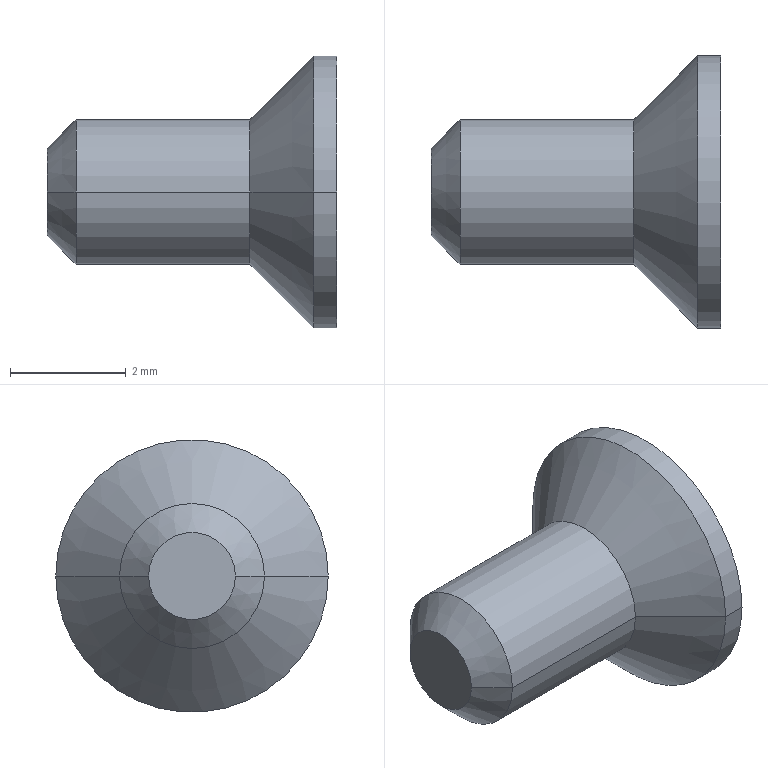Part | STEP file | ASND-0110-0219110001 | 1 solid | 26 faces | box 5 x 4.7 x 4.7 mm | volume 32.246 mm3 | cylinder 19 | cone 4 | plane 3 | commonest cylinder face diameters 0.4 x8 1.1 x7 2.5 x2 4.7 x2